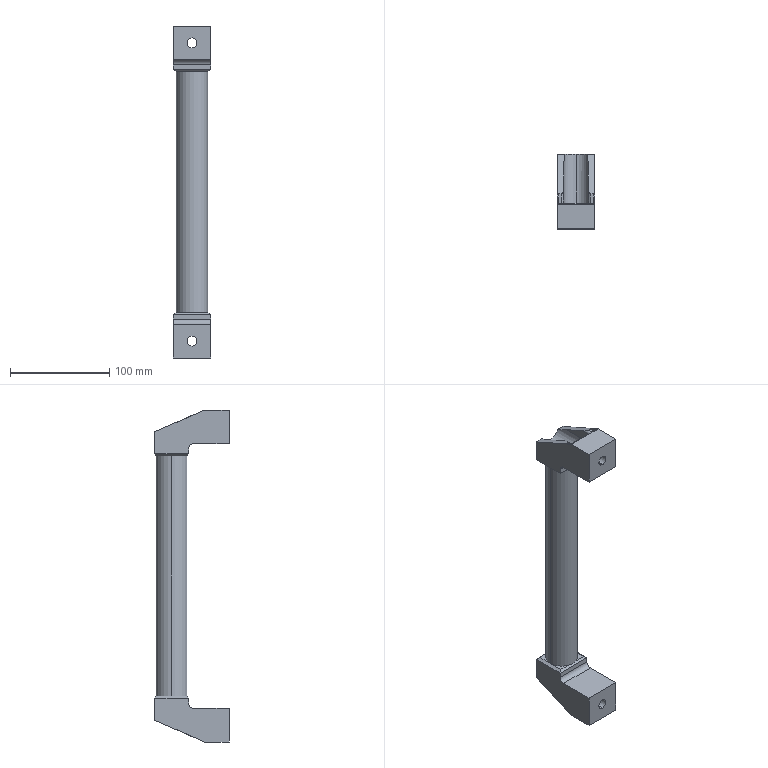Part | SolidWorks | features BaseBody 1 | 1 solid | 71 faces | box 38 x 75 x 334 mm | volume 331639 mm3 | plane 52 | cylinder 19 | commonest cylinder face diameters 10 x6 5 x4 16.5 x4 25 x3 32 x2